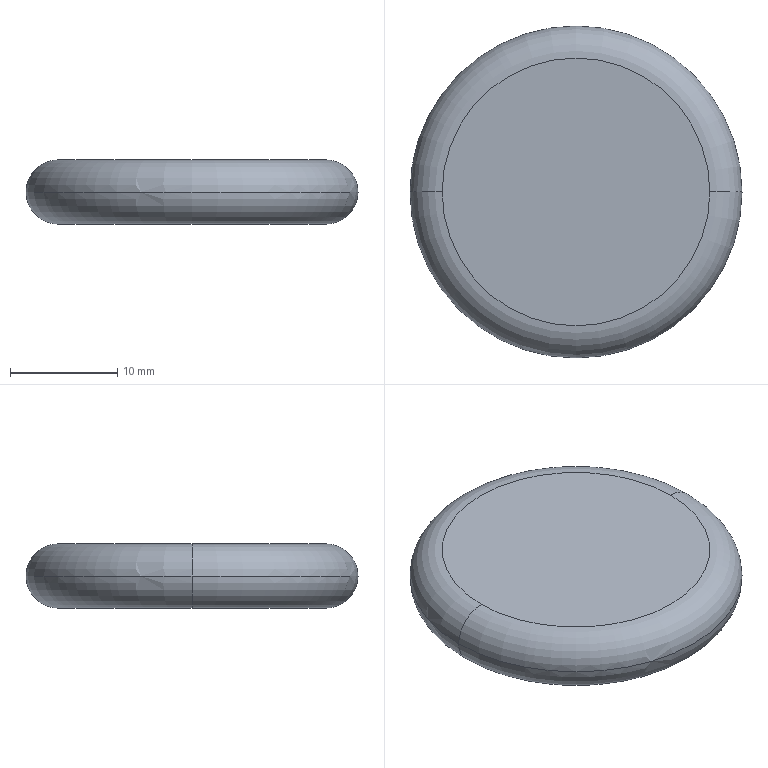Part | Creo | 1 solid | 6 faces | box 31 x 31 x 6 mm | volume 4169 mm3 | torus 4 | plane 2
STEP:
#1=CARTESIAN_POINT('',(12.5,0.,35.161));
#2=VERTEX_POINT('',#1);
#3=CARTESIAN_POINT('',(-12.5,0.,35.161));
#4=VERTEX_POINT('',#3);
#5=CARTESIAN_POINT('',(0.,0.,35.161));
#6=DIRECTION('',(0.,0.,-1.));
#7=DIRECTION('',(1.,0.,0.));
#8=AXIS2_PLACEMENT_3D('',#5,#6,#7);
#9=CIRCLE('',#8,12.5);
#10=EDGE_CURVE('',#2,#4,#9,.T.);
#11=ORIENTED_EDGE('',*,*,#10,.F.);
#12=CARTESIAN_POINT('',(0.,0.,35.161));
#13=DIRECTION('',(0.,0.,-1.));
#14=DIRECTION('',(-1.,0.,0.));
#15=AXIS2_PLACEMENT_3D('',#12,#13,#14);
#16=CIRCLE('',#15,12.5);
#17=EDGE_CURVE('',#4,#2,#16,.T.);
#18=ORIENTED_EDGE('',*,*,#17,.F.);
#19=EDGE_LOOP('',(#11,#18));
#20=FACE_OUTER_BOUND('',#19,.F.);
#21=CARTESIAN_POINT('',(0.,0.,35.161));
#22=DIRECTION('',(0.,0.,1.));
#23=DIRECTION('',(1.,0.,0.));
#24=AXIS2_PLACEMENT_3D('',#21,#22,#23);
#25=PLANE('',#24);
#26=ADVANCED_FACE('',(#20),#25,.F.);
#27=ORIENTED_EDGE('',*,*,#10,.T.);
#28=CARTESIAN_POINT('',(-15.5,0.,38.161));
#29=VERTEX_POINT('',#28);
#30=CARTESIAN_POINT('',(-12.5,0.,38.161));
#31=DIRECTION('',(0.,1.,0.));
#32=DIRECTION('',(0.,0.,-1.));
#33=AXIS2_PLACEMENT_3D('',#30,#31,#32);
#34=CIRCLE('',#33,3.);
#35=EDGE_CURVE('',#4,#29,#34,.T.);
#36=ORIENTED_EDGE('',*,*,#35,.T.);
#37=CARTESIAN_POINT('',(15.5,0.,38.161));
#38=VERTEX_POINT('',#37);
#39=CARTESIAN_POINT('',(0.,0.,38.161));
#40=DIRECTION('',(0.,0.,1.));
#41=DIRECTION('',(-1.,0.,0.));
#42=AXIS2_PLACEMENT_3D('',#39,#40,#41);
#43=CIRCLE('',#42,15.5);
#44=EDGE_CURVE('',#29,#38,#43,.T.);
#45=ORIENTED_EDGE('',*,*,#44,.T.);
#46=CARTESIAN_POINT('',(12.5,0.,38.161));
#47=DIRECTION('',(0.,-1.,0.));
#48=DIRECTION('',(0.,0.,-1.));
#49=AXIS2_PLACEMENT_3D('',#46,#47,#48);
#50=CIRCLE('',#49,3.);
#51=EDGE_CURVE('',#2,#38,#50,.T.);
#52=ORIENTED_EDGE('',*,*,#51,.F.);
#53=EDGE_LOOP('',(#27,#36,#45,#52));
#54=FACE_OUTER_BOUND('',#53,.F.);
#55=CARTESIAN_POINT('',(0.,0.,38.161));
#56=DIRECTION('',(0.,0.,1.));
#57=DIRECTION('',(1.,0.,0.));
#58=AXIS2_PLACEMENT_3D('',#55,#56,#57);
#59=TOROIDAL_SURFACE('',#58,12.5,3.);
#60=ADVANCED_FACE('',(#54),#59,.T.);
#61=ORIENTED_EDGE('',*,*,#17,.T.);
#62=ORIENTED_EDGE('',*,*,#51,.T.);
#63=CARTESIAN_POINT('',(0.,0.,38.161));
#64=DIRECTION('',(0.,0.,1.));
#65=DIRECTION('',(1.,0.,0.));
#66=AXIS2_PLACEMENT_3D('',#63,#64,#65);
#67=CIRCLE('',#66,15.5);
#68=EDGE_CURVE('',#38,#29,#67,.T.);
#69=ORIENTED_EDGE('',*,*,#68,.T.);
#70=ORIENTED_EDGE('',*,*,#35,.F.);
#71=EDGE_LOOP('',(#61,#62,#69,#70));
#72=FACE_OUTER_BOUND('',#71,.F.);
#73=CARTESIAN_POINT('',(0.,0.,38.161));
#74=DIRECTION('',(0.,0.,1.));
#75=DIRECTION('',(1.,0.,0.));
#76=AXIS2_PLACEMENT_3D('',#73,#74,#75);
#77=TOROIDAL_SURFACE('',#76,12.5,3.);
#78=ADVANCED_FACE('',(#72),#77,.T.);
#79=CARTESIAN_POINT('',(12.5,0.,41.161));
#80=VERTEX_POINT('',#79);
#81=CARTESIAN_POINT('',(-12.5,0.,41.161));
#82=VERTEX_POINT('',#81);
#83=CARTESIAN_POINT('',(0.,0.,41.161));
#84=DIRECTION('',(0.,0.,1.));
#85=DIRECTION('',(1.,0.,0.));
#86=AXIS2_PLACEMENT_3D('',#83,#84,#85);
#87=CIRCLE('',#86,12.5);
#88=EDGE_CURVE('',#80,#82,#87,.T.);
#89=ORIENTED_EDGE('',*,*,#88,.T.);
#90=CARTESIAN_POINT('',(-12.5,0.,38.161));
#91=DIRECTION('',(0.,1.,0.));
#92=DIRECTION('',(-1.,0.,0.));
#93=AXIS2_PLACEMENT_3D('',#90,#91,#92);
#94=CIRCLE('',#93,3.);
#95=EDGE_CURVE('',#29,#82,#94,.T.);
#96=ORIENTED_EDGE('',*,*,#95,.F.);
#97=ORIENTED_EDGE('',*,*,#68,.F.);
#98=CARTESIAN_POINT('',(12.5,0.,38.161));
#99=DIRECTION('',(0.,-1.,0.));
#100=DIRECTION('',(1.,0.,0.));
#101=AXIS2_PLACEMENT_3D('',#98,#99,#100);
#102=CIRCLE('',#101,3.);
#103=EDGE_CURVE('',#38,#80,#102,.T.);
#104=ORIENTED_EDGE('',*,*,#103,.T.);
#105=EDGE_LOOP('',(#89,#96,#97,#104));
#106=FACE_OUTER_BOUND('',#105,.F.);
#107=CARTESIAN_POINT('',(0.,0.,38.161));
#108=DIRECTION('',(0.,0.,1.));
#109=DIRECTION('',(1.,0.,0.));
#110=AXIS2_PLACEMENT_3D('',#107,#108,#109);
#111=TOROIDAL_SURFACE('',#110,12.5,3.);
#112=ADVANCED_FACE('',(#106),#111,.T.);
#113=ORIENTED_EDGE('',*,*,#88,.F.);
#114=CARTESIAN_POINT('',(0.,0.,41.161));
#115=DIRECTION('',(0.,0.,1.));
#116=DIRECTION('',(-1.,0.,0.));
#117=AXIS2_PLACEMENT_3D('',#114,#115,#116);
#118=CIRCLE('',#117,12.5);
#119=EDGE_CURVE('',#82,#80,#118,.T.);
#120=ORIENTED_EDGE('',*,*,#119,.F.);
#121=EDGE_LOOP('',(#113,#120));
#122=FACE_OUTER_BOUND('',#121,.F.);
#123=CARTESIAN_POINT('',(0.,0.,41.161));
#124=DIRECTION('',(0.,0.,1.));
#125=DIRECTION('',(1.,0.,0.));
#126=AXIS2_PLACEMENT_3D('',#123,#124,#125);
#127=PLANE('',#126);
#128=ADVANCED_FACE('',(#122),#127,.T.);
#129=ORIENTED_EDGE('',*,*,#119,.T.);
#130=ORIENTED_EDGE('',*,*,#103,.F.);
#131=ORIENTED_EDGE('',*,*,#44,.F.);
#132=ORIENTED_EDGE('',*,*,#95,.T.);
#133=EDGE_LOOP('',(#129,#130,#131,#132));
#134=FACE_OUTER_BOUND('',#133,.F.);
#135=CARTESIAN_POINT('',(0.,0.,38.161));
#136=DIRECTION('',(0.,0.,1.));
#137=DIRECTION('',(1.,0.,0.));
#138=AXIS2_PLACEMENT_3D('',#135,#136,#137);
#139=TOROIDAL_SURFACE('',#138,12.5,3.);
#140=ADVANCED_FACE('',(#134),#139,.T.);
#141=CLOSED_SHELL('',(#26,#60,#78,#112,#128,#140));
#142=MANIFOLD_SOLID_BREP('',#141);
#143=(LENGTH_UNIT()NAMED_UNIT(*)SI_UNIT(.MILLI.,.METRE.));
#144=UNCERTAINTY_MEASURE_WITH_UNIT(LENGTH_MEASURE(0.004425),#143,'','');
#145=(NAMED_UNIT(*)PLANE_ANGLE_UNIT()SI_UNIT($,.RADIAN.));
#146=PLANE_ANGLE_MEASURE_WITH_UNIT(PLANE_ANGLE_MEASURE(0.01745),#145);
#147=(CONVERSION_BASED_UNIT('DEGREE',#146)NAMED_UNIT(*)PLANE_ANGLE_UNIT());
#148=(NAMED_UNIT(*)SI_UNIT($,.STERADIAN.)SOLID_ANGLE_UNIT());
#149=(GEOMETRIC_REPRESENTATION_CONTEXT(3)GLOBAL_UNCERTAINTY_ASSIGNED_CONTEXT((#144))GLOBAL_UNIT_ASSIGNED_CONTEXT((#143,#147,#148))REPRESENTATION_CONTEXT('',''));
#150=ADVANCED_BREP_SHAPE_REPRESENTATION('',(#142),#149);